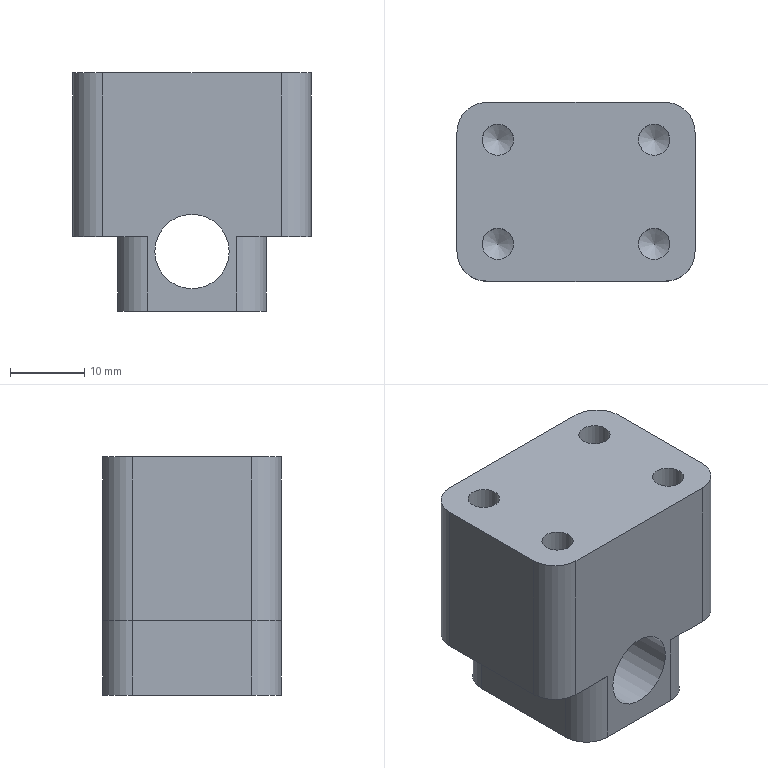Part | NX | features BREP 1, DATUM_CSYS 1 | 1 solid | 37 faces | box 32 x 24 x 32 mm | volume 18240 mm3 | cylinder 21 | plane 10 | cone 6 | commonest cylinder face diameters 4.2 x8 8 x8 2.5 x4 10 x1
STEP:
#1=CARTESIAN_POINT('',(12.,12.,5.));
#2=VERTEX_POINT('',#1);
#3=CARTESIAN_POINT('',(6.,12.,5.));
#4=VERTEX_POINT('',#3);
#5=CARTESIAN_POINT('',(12.,12.,5.));
#6=DIRECTION('',(-1.,0.,0.));
#7=VECTOR('',#6,1000.);
#8=LINE('',#5,#7);
#9=EDGE_CURVE('',#2,#4,#8,.T.);
#10=ORIENTED_EDGE('',*,*,#9,.T.);
#11=CARTESIAN_POINT('',(6.,12.,-5.));
#12=VERTEX_POINT('',#11);
#13=CARTESIAN_POINT('',(6.,12.,-5.));
#14=DIRECTION('',(0.,0.,1.));
#15=VECTOR('',#14,1000.);
#16=LINE('',#13,#15);
#17=EDGE_CURVE('',#12,#4,#16,.T.);
#18=ORIENTED_EDGE('',*,*,#17,.F.);
#19=CARTESIAN_POINT('',(-6.,12.,-5.));
#20=VERTEX_POINT('',#19);
#21=CARTESIAN_POINT('',(-6.,12.,-5.));
#22=DIRECTION('',(1.,0.,0.));
#23=VECTOR('',#22,1000.);
#24=LINE('',#21,#23);
#25=EDGE_CURVE('',#20,#12,#24,.T.);
#26=ORIENTED_EDGE('',*,*,#25,.F.);
#27=CARTESIAN_POINT('',(-6.,12.,5.));
#28=VERTEX_POINT('',#27);
#29=CARTESIAN_POINT('',(-6.,12.,5.));
#30=DIRECTION('',(0.,0.,-1.));
#31=VECTOR('',#30,1000.);
#32=LINE('',#29,#31);
#33=EDGE_CURVE('',#28,#20,#32,.T.);
#34=ORIENTED_EDGE('',*,*,#33,.F.);
#35=CARTESIAN_POINT('',(-12.,12.,5.));
#36=VERTEX_POINT('',#35);
#37=CARTESIAN_POINT('',(-12.,12.,5.));
#38=DIRECTION('',(1.,0.,0.));
#39=VECTOR('',#38,1000.);
#40=LINE('',#37,#39);
#41=EDGE_CURVE('',#36,#28,#40,.T.);
#42=ORIENTED_EDGE('',*,*,#41,.F.);
#43=CARTESIAN_POINT('',(-12.,12.,27.));
#44=VERTEX_POINT('',#43);
#45=CARTESIAN_POINT('',(-12.,12.,27.));
#46=DIRECTION('',(0.,0.,-1.));
#47=VECTOR('',#46,1000.);
#48=LINE('',#45,#47);
#49=EDGE_CURVE('',#44,#36,#48,.T.);
#50=ORIENTED_EDGE('',*,*,#49,.F.);
#51=CARTESIAN_POINT('',(12.,12.,27.));
#52=VERTEX_POINT('',#51);
#53=CARTESIAN_POINT('',(12.,12.,27.));
#54=DIRECTION('',(-1.,0.,0.));
#55=VECTOR('',#54,1000.);
#56=LINE('',#53,#55);
#57=EDGE_CURVE('',#52,#44,#56,.T.);
#58=ORIENTED_EDGE('',*,*,#57,.F.);
#59=CARTESIAN_POINT('',(12.,12.,5.));
#60=DIRECTION('',(0.,0.,1.));
#61=VECTOR('',#60,1000.);
#62=LINE('',#59,#61);
#63=EDGE_CURVE('',#2,#52,#62,.T.);
#64=ORIENTED_EDGE('',*,*,#63,.F.);
#65=EDGE_LOOP('',(#10,#18,#26,#34,#42,#50,#58,#64));
#66=FACE_BOUND('',#65,.T.);
#67=CARTESIAN_POINT('',(5.,12.,3.));
#68=VERTEX_POINT('',#67);
#69=CARTESIAN_POINT('',(0.,12.,3.));
#70=DIRECTION('',(0.,1.,0.));
#71=DIRECTION('',(1.,0.,0.));
#72=AXIS2_PLACEMENT_3D('',#69,#70,#71);
#73=CIRCLE('',#72,5.);
#74=EDGE_CURVE('',#68,#68,#73,.T.);
#75=ORIENTED_EDGE('',*,*,#74,.F.);
#76=EDGE_LOOP('',(#75));
#77=FACE_BOUND('',#76,.T.);
#78=CARTESIAN_POINT('',(0.,12.,11.));
#79=DIRECTION('',(0.,-1.,0.));
#80=DIRECTION('',(-1.,0.,0.));
#81=AXIS2_PLACEMENT_3D('',#78,#79,#80);
#82=PLANE('',#81);
#83=ADVANCED_FACE('',(#66,#77),#82,.F.);
#84=CARTESIAN_POINT('',(12.,-12.,5.));
#85=VERTEX_POINT('',#84);
#86=CARTESIAN_POINT('',(12.,-12.,27.));
#87=VERTEX_POINT('',#86);
#88=CARTESIAN_POINT('',(12.,-12.,5.));
#89=DIRECTION('',(0.,0.,1.));
#90=VECTOR('',#89,1000.);
#91=LINE('',#88,#90);
#92=EDGE_CURVE('',#85,#87,#91,.T.);
#93=ORIENTED_EDGE('',*,*,#92,.T.);
#94=CARTESIAN_POINT('',(-12.,-12.,27.));
#95=VERTEX_POINT('',#94);
#96=CARTESIAN_POINT('',(12.,-12.,27.));
#97=DIRECTION('',(-1.,0.,0.));
#98=VECTOR('',#97,1000.);
#99=LINE('',#96,#98);
#100=EDGE_CURVE('',#87,#95,#99,.T.);
#101=ORIENTED_EDGE('',*,*,#100,.T.);
#102=CARTESIAN_POINT('',(-12.,-12.,5.));
#103=VERTEX_POINT('',#102);
#104=CARTESIAN_POINT('',(-12.,-12.,27.));
#105=DIRECTION('',(0.,0.,-1.));
#106=VECTOR('',#105,1000.);
#107=LINE('',#104,#106);
#108=EDGE_CURVE('',#95,#103,#107,.T.);
#109=ORIENTED_EDGE('',*,*,#108,.T.);
#110=CARTESIAN_POINT('',(-6.,-12.,5.));
#111=VERTEX_POINT('',#110);
#112=CARTESIAN_POINT('',(-12.,-12.,5.));
#113=DIRECTION('',(1.,0.,0.));
#114=VECTOR('',#113,1000.);
#115=LINE('',#112,#114);
#116=EDGE_CURVE('',#103,#111,#115,.T.);
#117=ORIENTED_EDGE('',*,*,#116,.T.);
#118=CARTESIAN_POINT('',(-6.,-12.,-5.));
#119=VERTEX_POINT('',#118);
#120=CARTESIAN_POINT('',(-6.,-12.,5.));
#121=DIRECTION('',(0.,0.,-1.));
#122=VECTOR('',#121,1000.);
#123=LINE('',#120,#122);
#124=EDGE_CURVE('',#111,#119,#123,.T.);
#125=ORIENTED_EDGE('',*,*,#124,.T.);
#126=CARTESIAN_POINT('',(6.,-12.,-5.));
#127=VERTEX_POINT('',#126);
#128=CARTESIAN_POINT('',(-6.,-12.,-5.));
#129=DIRECTION('',(1.,0.,0.));
#130=VECTOR('',#129,1000.);
#131=LINE('',#128,#130);
#132=EDGE_CURVE('',#119,#127,#131,.T.);
#133=ORIENTED_EDGE('',*,*,#132,.T.);
#134=CARTESIAN_POINT('',(6.,-12.,5.));
#135=VERTEX_POINT('',#134);
#136=CARTESIAN_POINT('',(6.,-12.,-5.));
#137=DIRECTION('',(0.,0.,1.));
#138=VECTOR('',#137,1000.);
#139=LINE('',#136,#138);
#140=EDGE_CURVE('',#127,#135,#139,.T.);
#141=ORIENTED_EDGE('',*,*,#140,.T.);
#142=CARTESIAN_POINT('',(12.,-12.,5.));
#143=DIRECTION('',(-1.,0.,0.));
#144=VECTOR('',#143,1000.);
#145=LINE('',#142,#144);
#146=EDGE_CURVE('',#85,#135,#145,.T.);
#147=ORIENTED_EDGE('',*,*,#146,.F.);
#148=EDGE_LOOP('',(#93,#101,#109,#117,#125,#133,#141,#147));
#149=FACE_BOUND('',#148,.T.);
#150=CARTESIAN_POINT('',(5.,-12.,3.));
#151=VERTEX_POINT('',#150);
#152=CARTESIAN_POINT('',(0.,-12.,3.));
#153=DIRECTION('',(0.,1.,0.));
#154=DIRECTION('',(1.,0.,0.));
#155=AXIS2_PLACEMENT_3D('',#152,#153,#154);
#156=CIRCLE('',#155,5.);
#157=EDGE_CURVE('',#151,#151,#156,.T.);
#158=ORIENTED_EDGE('',*,*,#157,.T.);
#159=EDGE_LOOP('',(#158));
#160=FACE_BOUND('',#159,.T.);
#161=CARTESIAN_POINT('',(0.,-12.,11.));
#162=DIRECTION('',(0.,-1.,0.));
#163=DIRECTION('',(-1.,0.,0.));
#164=AXIS2_PLACEMENT_3D('',#161,#162,#163);
#165=PLANE('',#164);
#166=ADVANCED_FACE('',(#149,#160),#165,.T.);
#167=ORIENTED_EDGE('',*,*,#25,.T.);
#168=CARTESIAN_POINT('',(10.,8.,-5.));
#169=VERTEX_POINT('',#168);
#170=CARTESIAN_POINT('',(6.,8.,-5.));
#171=DIRECTION('',(0.,0.,-1.));
#172=DIRECTION('',(0.,1.,0.));
#173=AXIS2_PLACEMENT_3D('',#170,#171,#172);
#174=CIRCLE('',#173,4.);
#175=EDGE_CURVE('',#12,#169,#174,.T.);
#176=ORIENTED_EDGE('',*,*,#175,.T.);
#177=CARTESIAN_POINT('',(10.,-8.,-5.));
#178=VERTEX_POINT('',#177);
#179=CARTESIAN_POINT('',(10.,8.,-5.));
#180=DIRECTION('',(0.,-1.,0.));
#181=VECTOR('',#180,1000.);
#182=LINE('',#179,#181);
#183=EDGE_CURVE('',#169,#178,#182,.T.);
#184=ORIENTED_EDGE('',*,*,#183,.T.);
#185=CARTESIAN_POINT('',(6.,-8.,-5.));
#186=DIRECTION('',(0.,0.,1.));
#187=DIRECTION('',(0.,-1.,0.));
#188=AXIS2_PLACEMENT_3D('',#185,#186,#187);
#189=CIRCLE('',#188,4.);
#190=EDGE_CURVE('',#127,#178,#189,.T.);
#191=ORIENTED_EDGE('',*,*,#190,.F.);
#192=ORIENTED_EDGE('',*,*,#132,.F.);
#193=CARTESIAN_POINT('',(-10.,-8.,-5.));
#194=VERTEX_POINT('',#193);
#195=CARTESIAN_POINT('',(-6.,-8.,-5.));
#196=DIRECTION('',(0.,0.,-1.));
#197=DIRECTION('',(0.,-1.,0.));
#198=AXIS2_PLACEMENT_3D('',#195,#196,#197);
#199=CIRCLE('',#198,4.);
#200=EDGE_CURVE('',#119,#194,#199,.T.);
#201=ORIENTED_EDGE('',*,*,#200,.T.);
#202=CARTESIAN_POINT('',(-10.,8.,-5.));
#203=VERTEX_POINT('',#202);
#204=CARTESIAN_POINT('',(-10.,8.,-5.));
#205=DIRECTION('',(0.,-1.,0.));
#206=VECTOR('',#205,1000.);
#207=LINE('',#204,#206);
#208=EDGE_CURVE('',#203,#194,#207,.T.);
#209=ORIENTED_EDGE('',*,*,#208,.F.);
#210=CARTESIAN_POINT('',(-6.,8.,-5.));
#211=DIRECTION('',(0.,0.,1.));
#212=DIRECTION('',(0.,1.,0.));
#213=AXIS2_PLACEMENT_3D('',#210,#211,#212);
#214=CIRCLE('',#213,4.);
#215=EDGE_CURVE('',#20,#203,#214,.T.);
#216=ORIENTED_EDGE('',*,*,#215,.F.);
#217=EDGE_LOOP('',(#167,#176,#184,#191,#192,#201,#209,#216));
#218=FACE_BOUND('',#217,.T.);
#219=CARTESIAN_POINT('',(8.75,0.,-5.));
#220=VERTEX_POINT('',#219);
#221=CARTESIAN_POINT('',(7.5,0.,-5.));
#222=DIRECTION('',(0.,0.,1.));
#223=DIRECTION('',(1.,0.,0.));
#224=AXIS2_PLACEMENT_3D('',#221,#222,#223);
#225=CIRCLE('',#224,1.25);
#226=EDGE_CURVE('',#220,#220,#225,.T.);
#227=ORIENTED_EDGE('',*,*,#226,.T.);
#228=EDGE_LOOP('',(#227));
#229=FACE_BOUND('',#228,.T.);
#230=CARTESIAN_POINT('',(-6.25,0.,-5.));
#231=VERTEX_POINT('',#230);
#232=CARTESIAN_POINT('',(-7.5,0.,-5.));
#233=DIRECTION('',(0.,0.,1.));
#234=DIRECTION('',(1.,0.,0.));
#235=AXIS2_PLACEMENT_3D('',#232,#233,#234);
#236=CIRCLE('',#235,1.25);
#237=EDGE_CURVE('',#231,#231,#236,.T.);
#238=ORIENTED_EDGE('',*,*,#237,.T.);
#239=EDGE_LOOP('',(#238));
#240=FACE_BOUND('',#239,.T.);
#241=CARTESIAN_POINT('',(0.,0.,-5.));
#242=DIRECTION('',(0.,0.,-1.));
#243=DIRECTION('',(-1.,0.,0.));
#244=AXIS2_PLACEMENT_3D('',#241,#242,#243);
#245=PLANE('',#244);
#246=ADVANCED_FACE('',(#218,#229,#240),#245,.T.);
#247=ORIENTED_EDGE('',*,*,#183,.F.);
#248=CARTESIAN_POINT('',(10.,8.,5.));
#249=VERTEX_POINT('',#248);
#250=CARTESIAN_POINT('',(10.,8.,-5.));
#251=DIRECTION('',(0.,0.,1.));
#252=VECTOR('',#251,1000.);
#253=LINE('',#250,#252);
#254=EDGE_CURVE('',#169,#249,#253,.T.);
#255=ORIENTED_EDGE('',*,*,#254,.T.);
#256=CARTESIAN_POINT('',(10.,-8.,5.));
#257=VERTEX_POINT('',#256);
#258=CARTESIAN_POINT('',(10.,8.,5.));
#259=DIRECTION('',(0.,-1.,0.));
#260=VECTOR('',#259,1000.);
#261=LINE('',#258,#260);
#262=EDGE_CURVE('',#249,#257,#261,.T.);
#263=ORIENTED_EDGE('',*,*,#262,.T.);
#264=CARTESIAN_POINT('',(10.,-8.,-5.));
#265=DIRECTION('',(0.,0.,1.));
#266=VECTOR('',#265,1000.);
#267=LINE('',#264,#266);
#268=EDGE_CURVE('',#178,#257,#267,.T.);
#269=ORIENTED_EDGE('',*,*,#268,.F.);
#270=EDGE_LOOP('',(#247,#255,#263,#269));
#271=FACE_BOUND('',#270,.T.);
#272=CARTESIAN_POINT('',(10.,0.,0.));
#273=DIRECTION('',(1.,0.,0.));
#274=DIRECTION('',(0.,0.,-1.));
#275=AXIS2_PLACEMENT_3D('',#272,#273,#274);
#276=PLANE('',#275);
#277=ADVANCED_FACE('',(#271),#276,.T.);
#278=CARTESIAN_POINT('',(16.,8.,5.));
#279=VERTEX_POINT('',#278);
#280=CARTESIAN_POINT('',(12.,8.,5.));
#281=DIRECTION('',(0.,0.,-1.));
#282=DIRECTION('',(0.,1.,0.));
#283=AXIS2_PLACEMENT_3D('',#280,#281,#282);
#284=CIRCLE('',#283,4.);
#285=EDGE_CURVE('',#2,#279,#284,.T.);
#286=ORIENTED_EDGE('',*,*,#285,.T.);
#287=CARTESIAN_POINT('',(16.,-8.,5.));
#288=VERTEX_POINT('',#287);
#289=CARTESIAN_POINT('',(16.,8.,5.));
#290=DIRECTION('',(0.,-1.,0.));
#291=VECTOR('',#290,1000.);
#292=LINE('',#289,#291);
#293=EDGE_CURVE('',#279,#288,#292,.T.);
#294=ORIENTED_EDGE('',*,*,#293,.T.);
#295=CARTESIAN_POINT('',(12.,-8.,5.));
#296=DIRECTION('',(0.,0.,1.));
#297=DIRECTION('',(0.,-1.,0.));
#298=AXIS2_PLACEMENT_3D('',#295,#296,#297);
#299=CIRCLE('',#298,4.);
#300=EDGE_CURVE('',#85,#288,#299,.T.);
#301=ORIENTED_EDGE('',*,*,#300,.F.);
#302=ORIENTED_EDGE('',*,*,#146,.T.);
#303=CARTESIAN_POINT('',(6.,-8.,5.));
#304=DIRECTION('',(0.,0.,-1.));
#305=DIRECTION('',(1.,0.,0.));
#306=AXIS2_PLACEMENT_3D('',#303,#304,#305);
#307=CIRCLE('',#306,4.);
#308=EDGE_CURVE('',#257,#135,#307,.T.);
#309=ORIENTED_EDGE('',*,*,#308,.F.);
#310=ORIENTED_EDGE('',*,*,#262,.F.);
#311=CARTESIAN_POINT('',(6.,8.,5.));
#312=DIRECTION('',(0.,0.,1.));
#313=DIRECTION('',(1.,0.,0.));
#314=AXIS2_PLACEMENT_3D('',#311,#312,#313);
#315=CIRCLE('',#314,4.);
#316=EDGE_CURVE('',#249,#4,#315,.T.);
#317=ORIENTED_EDGE('',*,*,#316,.T.);
#318=ORIENTED_EDGE('',*,*,#9,.F.);
#319=EDGE_LOOP('',(#286,#294,#301,#302,#309,#310,#317,#318));
#320=FACE_BOUND('',#319,.T.);
#321=CARTESIAN_POINT('',(11.,0.,5.));
#322=DIRECTION('',(0.,0.,-1.));
#323=DIRECTION('',(-1.,0.,0.));
#324=AXIS2_PLACEMENT_3D('',#321,#322,#323);
#325=PLANE('',#324);
#326=ADVANCED_FACE('',(#320),#325,.T.);
#327=ORIENTED_EDGE('',*,*,#293,.F.);
#328=CARTESIAN_POINT('',(16.,8.,27.));
#329=VERTEX_POINT('',#328);
#330=CARTESIAN_POINT('',(16.,8.,5.));
#331=DIRECTION('',(0.,0.,1.));
#332=VECTOR('',#331,1000.);
#333=LINE('',#330,#332);
#334=EDGE_CURVE('',#279,#329,#333,.T.);
#335=ORIENTED_EDGE('',*,*,#334,.T.);
#336=CARTESIAN_POINT('',(16.,-8.,27.));
#337=VERTEX_POINT('',#336);
#338=CARTESIAN_POINT('',(16.,8.,27.));
#339=DIRECTION('',(0.,-1.,0.));
#340=VECTOR('',#339,1000.);
#341=LINE('',#338,#340);
#342=EDGE_CURVE('',#329,#337,#341,.T.);
#343=ORIENTED_EDGE('',*,*,#342,.T.);
#344=CARTESIAN_POINT('',(16.,-8.,5.));
#345=DIRECTION('',(0.,0.,1.));
#346=VECTOR('',#345,1000.);
#347=LINE('',#344,#346);
#348=EDGE_CURVE('',#288,#337,#347,.T.);
#349=ORIENTED_EDGE('',*,*,#348,.F.);
#350=EDGE_LOOP('',(#327,#335,#343,#349));
#351=FACE_BOUND('',#350,.T.);
#352=CARTESIAN_POINT('',(16.,0.,16.));
#353=DIRECTION('',(1.,0.,0.));
#354=DIRECTION('',(0.,0.,-1.));
#355=AXIS2_PLACEMENT_3D('',#352,#353,#354);
#356=PLANE('',#355);
#357=ADVANCED_FACE('',(#351),#356,.T.);
#358=CARTESIAN_POINT('',(-16.,8.,27.));
#359=VERTEX_POINT('',#358);
#360=CARTESIAN_POINT('',(-16.,-8.,27.));
#361=VERTEX_POINT('',#360);
#362=CARTESIAN_POINT('',(-16.,8.,27.));
#363=DIRECTION('',(0.,-1.,0.));
#364=VECTOR('',#363,1000.);
#365=LINE('',#362,#364);
#366=EDGE_CURVE('',#359,#361,#365,.T.);
#367=ORIENTED_EDGE('',*,*,#366,.F.);
#368=CARTESIAN_POINT('',(-16.,8.,5.));
#369=VERTEX_POINT('',#368);
#370=CARTESIAN_POINT('',(-16.,8.,27.));
#371=DIRECTION('',(0.,0.,-1.));
#372=VECTOR('',#371,1000.);
#373=LINE('',#370,#372);
#374=EDGE_CURVE('',#359,#369,#373,.T.);
#375=ORIENTED_EDGE('',*,*,#374,.T.);
#376=CARTESIAN_POINT('',(-16.,-8.,5.));
#377=VERTEX_POINT('',#376);
#378=CARTESIAN_POINT('',(-16.,8.,5.));
#379=DIRECTION('',(0.,-1.,0.));
#380=VECTOR('',#379,1000.);
#381=LINE('',#378,#380);
#382=EDGE_CURVE('',#369,#377,#381,.T.);
#383=ORIENTED_EDGE('',*,*,#382,.T.);
#384=CARTESIAN_POINT('',(-16.,-8.,27.));
#385=DIRECTION('',(0.,0.,-1.));
#386=VECTOR('',#385,1000.);
#387=LINE('',#384,#386);
#388=EDGE_CURVE('',#361,#377,#387,.T.);
#389=ORIENTED_EDGE('',*,*,#388,.F.);
#390=EDGE_LOOP('',(#367,#375,#383,#389));
#391=FACE_BOUND('',#390,.T.);
#392=CARTESIAN_POINT('',(-16.,0.,16.));
#393=DIRECTION('',(-1.,0.,0.));
#394=DIRECTION('',(0.,0.,1.));
#395=AXIS2_PLACEMENT_3D('',#392,#393,#394);
#396=PLANE('',#395);
#397=ADVANCED_FACE('',(#391),#396,.T.);
#398=CARTESIAN_POINT('',(-12.,-8.,5.));
#399=DIRECTION('',(0.,0.,-1.));
#400=DIRECTION('',(0.,-1.,0.));
#401=AXIS2_PLACEMENT_3D('',#398,#399,#400);
#402=CIRCLE('',#401,4.);
#403=EDGE_CURVE('',#103,#377,#402,.T.);
#404=ORIENTED_EDGE('',*,*,#403,.T.);
#405=ORIENTED_EDGE('',*,*,#382,.F.);
#406=CARTESIAN_POINT('',(-12.,8.,5.));
#407=DIRECTION('',(0.,0.,1.));
#408=DIRECTION('',(0.,1.,0.));
#409=AXIS2_PLACEMENT_3D('',#406,#407,#408);
#410=CIRCLE('',#409,4.);
#411=EDGE_CURVE('',#36,#369,#410,.T.);
#412=ORIENTED_EDGE('',*,*,#411,.F.);
#413=ORIENTED_EDGE('',*,*,#41,.T.);
#414=CARTESIAN_POINT('',(-10.,8.,5.));
#415=VERTEX_POINT('',#414);
#416=CARTESIAN_POINT('',(-6.,8.,5.));
#417=DIRECTION('',(0.,0.,-1.));
#418=DIRECTION('',(-1.,0.,0.));
#419=AXIS2_PLACEMENT_3D('',#416,#417,#418);
#420=CIRCLE('',#419,4.);
#421=EDGE_CURVE('',#415,#28,#420,.T.);
#422=ORIENTED_EDGE('',*,*,#421,.F.);
#423=CARTESIAN_POINT('',(-10.,-8.,5.));
#424=VERTEX_POINT('',#423);
#425=CARTESIAN_POINT('',(-10.,8.,5.));
#426=DIRECTION('',(0.,-1.,0.));
#427=VECTOR('',#426,1000.);
#428=LINE('',#425,#427);
#429=EDGE_CURVE('',#415,#424,#428,.T.);
#430=ORIENTED_EDGE('',*,*,#429,.T.);
#431=CARTESIAN_POINT('',(-6.,-8.,5.));
#432=DIRECTION('',(0.,0.,1.));
#433=DIRECTION('',(-1.,0.,0.));
#434=AXIS2_PLACEMENT_3D('',#431,#432,#433);
#435=CIRCLE('',#434,4.);
#436=EDGE_CURVE('',#424,#111,#435,.T.);
#437=ORIENTED_EDGE('',*,*,#436,.T.);
#438=ORIENTED_EDGE('',*,*,#116,.F.);
#439=EDGE_LOOP('',(#404,#405,#412,#413,#422,#430,#437,#438));
#440=FACE_BOUND('',#439,.T.);
#441=CARTESIAN_POINT('',(-11.,0.,5.));
#442=DIRECTION('',(0.,0.,-1.));
#443=DIRECTION('',(-1.,0.,0.));
#444=AXIS2_PLACEMENT_3D('',#441,#442,#443);
#445=PLANE('',#444);
#446=ADVANCED_FACE('',(#440),#445,.T.);
#447=ORIENTED_EDGE('',*,*,#429,.F.);
#448=CARTESIAN_POINT('',(-10.,8.,5.));
#449=DIRECTION('',(0.,0.,-1.));
#450=VECTOR('',#449,1000.);
#451=LINE('',#448,#450);
#452=EDGE_CURVE('',#415,#203,#451,.T.);
#453=ORIENTED_EDGE('',*,*,#452,.T.);
#454=ORIENTED_EDGE('',*,*,#208,.T.);
#455=CARTESIAN_POINT('',(-10.,-8.,5.));
#456=DIRECTION('',(0.,0.,-1.));
#457=VECTOR('',#456,1000.);
#458=LINE('',#455,#457);
#459=EDGE_CURVE('',#424,#194,#458,.T.);
#460=ORIENTED_EDGE('',*,*,#459,.F.);
#461=EDGE_LOOP('',(#447,#453,#454,#460));
#462=FACE_BOUND('',#461,.T.);
#463=CARTESIAN_POINT('',(-10.,0.,0.));
#464=DIRECTION('',(-1.,0.,0.));
#465=DIRECTION('',(0.,0.,1.));
#466=AXIS2_PLACEMENT_3D('',#463,#464,#465);
#467=PLANE('',#466);
#468=ADVANCED_FACE('',(#462),#467,.T.);
#469=CARTESIAN_POINT('',(12.,-8.,27.));
#470=DIRECTION('',(0.,0.,1.));
#471=DIRECTION('',(0.,-1.,0.));
#472=AXIS2_PLACEMENT_3D('',#469,#470,#471);
#473=CIRCLE('',#472,4.);
#474=EDGE_CURVE('',#87,#337,#473,.T.);
#475=ORIENTED_EDGE('',*,*,#474,.F.);
#476=ORIENTED_EDGE('',*,*,#92,.F.);
#477=ORIENTED_EDGE('',*,*,#300,.T.);
#478=ORIENTED_EDGE('',*,*,#348,.T.);
#479=EDGE_LOOP('',(#475,#476,#477,#478));
#480=FACE_BOUND('',#479,.T.);
#481=CARTESIAN_POINT('',(12.,-8.,-6.117));
#482=DIRECTION('',(0.,0.,1.));
#483=DIRECTION('',(0.,1.,0.));
#484=AXIS2_PLACEMENT_3D('',#481,#482,#483);
#485=CYLINDRICAL_SURFACE('',#484,4.);
#486=ADVANCED_FACE('',(#480),#485,.T.);
#487=CARTESIAN_POINT('',(-12.,-8.,27.));
#488=DIRECTION('',(0.,0.,-1.));
#489=DIRECTION('',(0.,-1.,0.));
#490=AXIS2_PLACEMENT_3D('',#487,#488,#489);
#491=CIRCLE('',#490,4.);
#492=EDGE_CURVE('',#95,#361,#491,.T.);
#493=ORIENTED_EDGE('',*,*,#492,.T.);
#494=ORIENTED_EDGE('',*,*,#388,.T.);
#495=ORIENTED_EDGE('',*,*,#403,.F.);
#496=ORIENTED_EDGE('',*,*,#108,.F.);
#497=EDGE_LOOP('',(#493,#494,#495,#496));
#498=FACE_BOUND('',#497,.T.);
#499=CARTESIAN_POINT('',(-12.,-8.,27.));
#500=DIRECTION('',(0.,0.,-1.));
#501=DIRECTION('',(0.,1.,0.));
#502=AXIS2_PLACEMENT_3D('',#499,#500,#501);
#503=CYLINDRICAL_SURFACE('',#502,4.);
#504=ADVANCED_FACE('',(#498),#503,.T.);
#505=ORIENTED_EDGE('',*,*,#334,.F.);
#506=ORIENTED_EDGE('',*,*,#285,.F.);
#507=ORIENTED_EDGE('',*,*,#63,.T.);
#508=CARTESIAN_POINT('',(12.,8.,27.));
#509=DIRECTION('',(0.,0.,-1.));
#510=DIRECTION('',(0.,1.,0.));
#511=AXIS2_PLACEMENT_3D('',#508,#509,#510);
#512=CIRCLE('',#511,4.);
#513=EDGE_CURVE('',#52,#329,#512,.T.);
#514=ORIENTED_EDGE('',*,*,#513,.T.);
#515=EDGE_LOOP('',(#505,#506,#507,#514));
#516=FACE_BOUND('',#515,.T.);
#517=CARTESIAN_POINT('',(12.,8.,-6.6));
#518=DIRECTION('',(0.,0.,1.));
#519=DIRECTION('',(0.,-1.,0.));
#520=AXIS2_PLACEMENT_3D('',#517,#518,#519);
#521=CYLINDRICAL_SURFACE('',#520,4.);
#522=ADVANCED_FACE('',(#516),#521,.T.);
#523=ORIENTED_EDGE('',*,*,#49,.T.);
#524=ORIENTED_EDGE('',*,*,#411,.T.);
#525=ORIENTED_EDGE('',*,*,#374,.F.);
#526=CARTESIAN_POINT('',(-12.,8.,27.));
#527=DIRECTION('',(0.,0.,1.));
#528=DIRECTION('',(0.,1.,0.));
#529=AXIS2_PLACEMENT_3D('',#526,#527,#528);
#530=CIRCLE('',#529,4.);
#531=EDGE_CURVE('',#44,#359,#530,.T.);
#532=ORIENTED_EDGE('',*,*,#531,.F.);
#533=EDGE_LOOP('',(#523,#524,#525,#532));
#534=FACE_BOUND('',#533,.T.);
#535=CARTESIAN_POINT('',(-12.,8.,27.));
#536=DIRECTION('',(0.,0.,-1.));
#537=DIRECTION('',(0.,-1.,0.));
#538=AXIS2_PLACEMENT_3D('',#535,#536,#537);
#539=CYLINDRICAL_SURFACE('',#538,4.);
#540=ADVANCED_FACE('',(#534),#539,.T.);
#541=ORIENTED_EDGE('',*,*,#452,.F.);
#542=ORIENTED_EDGE('',*,*,#421,.T.);
#543=ORIENTED_EDGE('',*,*,#33,.T.);
#544=ORIENTED_EDGE('',*,*,#215,.T.);
#545=EDGE_LOOP('',(#541,#542,#543,#544));
#546=FACE_BOUND('',#545,.T.);
#547=CARTESIAN_POINT('',(-6.,8.,28.175));
#548=DIRECTION('',(0.,0.,-1.));
#549=DIRECTION('',(0.,-1.,0.));
#550=AXIS2_PLACEMENT_3D('',#547,#548,#549);
#551=CYLINDRICAL_SURFACE('',#550,4.);
#552=ADVANCED_FACE('',(#546),#551,.T.);
#553=ORIENTED_EDGE('',*,*,#17,.T.);
#554=ORIENTED_EDGE('',*,*,#316,.F.);
#555=ORIENTED_EDGE('',*,*,#254,.F.);
#556=ORIENTED_EDGE('',*,*,#175,.F.);
#557=EDGE_LOOP('',(#553,#554,#555,#556));
#558=FACE_BOUND('',#557,.T.);
#559=CARTESIAN_POINT('',(6.,8.,-5.));
#560=DIRECTION('',(0.,0.,1.));
#561=DIRECTION('',(0.,-1.,0.));
#562=AXIS2_PLACEMENT_3D('',#559,#560,#561);
#563=CYLINDRICAL_SURFACE('',#562,4.);
#564=ADVANCED_FACE('',(#558),#563,.T.);
#565=ORIENTED_EDGE('',*,*,#190,.T.);
#566=ORIENTED_EDGE('',*,*,#268,.T.);
#567=ORIENTED_EDGE('',*,*,#308,.T.);
#568=ORIENTED_EDGE('',*,*,#140,.F.);
#569=EDGE_LOOP('',(#565,#566,#567,#568));
#570=FACE_BOUND('',#569,.T.);
#571=CARTESIAN_POINT('',(6.,-8.,-5.));
#572=DIRECTION('',(0.,0.,1.));
#573=DIRECTION('',(0.,1.,0.));
#574=AXIS2_PLACEMENT_3D('',#571,#572,#573);
#575=CYLINDRICAL_SURFACE('',#574,4.);
#576=ADVANCED_FACE('',(#570),#575,.T.);
#577=ORIENTED_EDGE('',*,*,#200,.F.);
#578=ORIENTED_EDGE('',*,*,#124,.F.);
#579=ORIENTED_EDGE('',*,*,#436,.F.);
#580=ORIENTED_EDGE('',*,*,#459,.T.);
#581=EDGE_LOOP('',(#577,#578,#579,#580));
#582=FACE_BOUND('',#581,.T.);
#583=CARTESIAN_POINT('',(-6.,-8.,28.6));
#584=DIRECTION('',(0.,0.,-1.));
#585=DIRECTION('',(0.,1.,0.));
#586=AXIS2_PLACEMENT_3D('',#583,#584,#585);
#587=CYLINDRICAL_SURFACE('',#586,4.);
#588=ADVANCED_FACE('',(#582),#587,.T.);
#589=ORIENTED_EDGE('',*,*,#100,.F.);
#590=ORIENTED_EDGE('',*,*,#474,.T.);
#591=ORIENTED_EDGE('',*,*,#342,.F.);
#592=ORIENTED_EDGE('',*,*,#513,.F.);
#593=ORIENTED_EDGE('',*,*,#57,.T.);
#594=ORIENTED_EDGE('',*,*,#531,.T.);
#595=ORIENTED_EDGE('',*,*,#366,.T.);
#596=ORIENTED_EDGE('',*,*,#492,.F.);
#597=EDGE_LOOP('',(#589,#590,#591,#592,#593,#594,#595,#596));
#598=FACE_BOUND('',#597,.T.);
#599=CARTESIAN_POINT('',(-8.4,7.,27.));
#600=VERTEX_POINT('',#599);
#601=CARTESIAN_POINT('',(-10.5,7.,27.));
#602=DIRECTION('',(0.,0.,-1.));
#603=DIRECTION('',(1.,0.,0.));
#604=AXIS2_PLACEMENT_3D('',#601,#602,#603);
#605=CIRCLE('',#604,2.1);
#606=EDGE_CURVE('',#600,#600,#605,.T.);
#607=ORIENTED_EDGE('',*,*,#606,.T.);
#608=EDGE_LOOP('',(#607));
#609=FACE_BOUND('',#608,.T.);
#610=CARTESIAN_POINT('',(12.6,7.,27.));
#611=VERTEX_POINT('',#610);
#612=CARTESIAN_POINT('',(10.5,7.,27.));
#613=DIRECTION('',(0.,0.,-1.));
#614=DIRECTION('',(1.,0.,0.));
#615=AXIS2_PLACEMENT_3D('',#612,#613,#614);
#616=CIRCLE('',#615,2.1);
#617=EDGE_CURVE('',#611,#611,#616,.T.);
#618=ORIENTED_EDGE('',*,*,#617,.T.);
#619=EDGE_LOOP('',(#618));
#620=FACE_BOUND('',#619,.T.);
#621=CARTESIAN_POINT('',(12.6,-7.,27.));
#622=VERTEX_POINT('',#621);
#623=CARTESIAN_POINT('',(10.5,-7.,27.));
#624=DIRECTION('',(0.,0.,-1.));
#625=DIRECTION('',(1.,0.,0.));
#626=AXIS2_PLACEMENT_3D('',#623,#624,#625);
#627=CIRCLE('',#626,2.1);
#628=EDGE_CURVE('',#622,#622,#627,.T.);
#629=ORIENTED_EDGE('',*,*,#628,.T.);
#630=EDGE_LOOP('',(#629));
#631=FACE_BOUND('',#630,.T.);
#632=CARTESIAN_POINT('',(-8.4,-7.,27.));
#633=VERTEX_POINT('',#632);
#634=CARTESIAN_POINT('',(-10.5,-7.,27.));
#635=DIRECTION('',(0.,0.,-1.));
#636=DIRECTION('',(1.,0.,0.));
#637=AXIS2_PLACEMENT_3D('',#634,#635,#636);
#638=CIRCLE('',#637,2.1);
#639=EDGE_CURVE('',#633,#633,#638,.T.);
#640=ORIENTED_EDGE('',*,*,#639,.T.);
#641=EDGE_LOOP('',(#640));
#642=FACE_BOUND('',#641,.T.);
#643=CARTESIAN_POINT('',(0.,0.,27.));
#644=DIRECTION('',(0.,0.,1.));
#645=DIRECTION('',(1.,0.,0.));
#646=AXIS2_PLACEMENT_3D('',#643,#644,#645);
#647=PLANE('',#646);
#648=ADVANCED_FACE('',(#598,#609,#620,#631,#642),#647,.T.);
#649=CARTESIAN_POINT('',(-8.4,7.,11.));
#650=VERTEX_POINT('',#649);
#651=CARTESIAN_POINT('',(-8.4,7.,27.));
#652=DIRECTION('',(0.,0.,-1.));
#653=VECTOR('',#652,1000.);
#654=LINE('',#651,#653);
#655=EDGE_CURVE('',#600,#650,#654,.T.);
#656=ORIENTED_EDGE('',*,*,#655,.T.);
#657=CARTESIAN_POINT('',(-10.5,7.,11.));
#658=DIRECTION('',(0.,0.,-1.));
#659=DIRECTION('',(1.,0.,0.));
#660=AXIS2_PLACEMENT_3D('',#657,#658,#659);
#661=CIRCLE('',#660,2.1);
#662=EDGE_CURVE('',#650,#650,#661,.T.);
#663=ORIENTED_EDGE('',*,*,#662,.T.);
#664=ORIENTED_EDGE('',*,*,#655,.F.);
#665=ORIENTED_EDGE('',*,*,#606,.F.);
#666=EDGE_LOOP('',(#656,#663,#664,#665));
#667=FACE_BOUND('',#666,.T.);
#668=CARTESIAN_POINT('',(-10.5,7.,27.));
#669=DIRECTION('',(0.,0.,-1.));
#670=DIRECTION('',(-1.,0.,0.));
#671=AXIS2_PLACEMENT_3D('',#668,#669,#670);
#672=CYLINDRICAL_SURFACE('',#671,2.1);
#673=ADVANCED_FACE('',(#667),#672,.F.);
#674=CARTESIAN_POINT('',(12.6,7.,11.));
#675=VERTEX_POINT('',#674);
#676=CARTESIAN_POINT('',(12.6,7.,27.));
#677=DIRECTION('',(0.,0.,-1.));
#678=VECTOR('',#677,1000.);
#679=LINE('',#676,#678);
#680=EDGE_CURVE('',#611,#675,#679,.T.);
#681=ORIENTED_EDGE('',*,*,#680,.T.);
#682=CARTESIAN_POINT('',(10.5,7.,11.));
#683=DIRECTION('',(0.,0.,-1.));
#684=DIRECTION('',(1.,0.,0.));
#685=AXIS2_PLACEMENT_3D('',#682,#683,#684);
#686=CIRCLE('',#685,2.1);
#687=EDGE_CURVE('',#675,#675,#686,.T.);
#688=ORIENTED_EDGE('',*,*,#687,.T.);
#689=ORIENTED_EDGE('',*,*,#680,.F.);
#690=ORIENTED_EDGE('',*,*,#617,.F.);
#691=EDGE_LOOP('',(#681,#688,#689,#690));
#692=FACE_BOUND('',#691,.T.);
#693=CARTESIAN_POINT('',(10.5,7.,27.));
#694=DIRECTION('',(0.,0.,-1.));
#695=DIRECTION('',(-1.,0.,0.));
#696=AXIS2_PLACEMENT_3D('',#693,#694,#695);
#697=CYLINDRICAL_SURFACE('',#696,2.1);
#698=ADVANCED_FACE('',(#692),#697,.F.);
#699=CARTESIAN_POINT('',(12.6,-7.,11.));
#700=VERTEX_POINT('',#699);
#701=CARTESIAN_POINT('',(12.6,-7.,27.));
#702=DIRECTION('',(0.,0.,-1.));
#703=VECTOR('',#702,1000.);
#704=LINE('',#701,#703);
#705=EDGE_CURVE('',#622,#700,#704,.T.);
#706=ORIENTED_EDGE('',*,*,#705,.T.);
#707=CARTESIAN_POINT('',(10.5,-7.,11.));
#708=DIRECTION('',(0.,0.,-1.));
#709=DIRECTION('',(1.,0.,0.));
#710=AXIS2_PLACEMENT_3D('',#707,#708,#709);
#711=CIRCLE('',#710,2.1);
#712=EDGE_CURVE('',#700,#700,#711,.T.);
#713=ORIENTED_EDGE('',*,*,#712,.T.);
#714=ORIENTED_EDGE('',*,*,#705,.F.);
#715=ORIENTED_EDGE('',*,*,#628,.F.);
#716=EDGE_LOOP('',(#706,#713,#714,#715));
#717=FACE_BOUND('',#716,.T.);
#718=CARTESIAN_POINT('',(10.5,-7.,27.));
#719=DIRECTION('',(0.,0.,-1.));
#720=DIRECTION('',(-1.,0.,0.));
#721=AXIS2_PLACEMENT_3D('',#718,#719,#720);
#722=CYLINDRICAL_SURFACE('',#721,2.1);
#723=ADVANCED_FACE('',(#717),#722,.F.);
#724=CARTESIAN_POINT('',(-8.4,-7.,11.));
#725=VERTEX_POINT('',#724);
#726=CARTESIAN_POINT('',(-8.4,-7.,27.));
#727=DIRECTION('',(0.,0.,-1.));
#728=VECTOR('',#727,1000.);
#729=LINE('',#726,#728);
#730=EDGE_CURVE('',#633,#725,#729,.T.);
#731=ORIENTED_EDGE('',*,*,#730,.T.);
#732=CARTESIAN_POINT('',(-10.5,-7.,11.));
#733=DIRECTION('',(0.,0.,-1.));
#734=DIRECTION('',(1.,0.,0.));
#735=AXIS2_PLACEMENT_3D('',#732,#733,#734);
#736=CIRCLE('',#735,2.1);
#737=EDGE_CURVE('',#725,#725,#736,.T.);
#738=ORIENTED_EDGE('',*,*,#737,.T.);
#739=ORIENTED_EDGE('',*,*,#730,.F.);
#740=ORIENTED_EDGE('',*,*,#639,.F.);
#741=EDGE_LOOP('',(#731,#738,#739,#740));
#742=FACE_BOUND('',#741,.T.);
#743=CARTESIAN_POINT('',(-10.5,-7.,27.));
#744=DIRECTION('',(0.,0.,-1.));
#745=DIRECTION('',(-1.,0.,0.));
#746=AXIS2_PLACEMENT_3D('',#743,#744,#745);
#747=CYLINDRICAL_SURFACE('',#746,2.1);
#748=ADVANCED_FACE('',(#742),#747,.F.);
#749=CARTESIAN_POINT('',(-8.4,7.,9.));
#750=VERTEX_POINT('',#749);
#751=CARTESIAN_POINT('',(-8.4,7.,11.));
#752=DIRECTION('',(0.,0.,-1.));
#753=VECTOR('',#752,1000.);
#754=LINE('',#751,#753);
#755=EDGE_CURVE('',#650,#750,#754,.T.);
#756=ORIENTED_EDGE('',*,*,#755,.T.);
#757=CARTESIAN_POINT('',(-10.5,7.,9.));
#758=DIRECTION('',(0.,0.,-1.));
#759=DIRECTION('',(1.,0.,0.));
#760=AXIS2_PLACEMENT_3D('',#757,#758,#759);
#761=CIRCLE('',#760,2.1);
#762=EDGE_CURVE('',#750,#750,#761,.T.);
#763=ORIENTED_EDGE('',*,*,#762,.T.);
#764=ORIENTED_EDGE('',*,*,#755,.F.);
#765=ORIENTED_EDGE('',*,*,#662,.F.);
#766=EDGE_LOOP('',(#756,#763,#764,#765));
#767=FACE_BOUND('',#766,.T.);
#768=CARTESIAN_POINT('',(-10.5,7.,11.));
#769=DIRECTION('',(0.,0.,-1.));
#770=DIRECTION('',(-1.,0.,0.));
#771=AXIS2_PLACEMENT_3D('',#768,#769,#770);
#772=CYLINDRICAL_SURFACE('',#771,2.1);
#773=ADVANCED_FACE('',(#767),#772,.F.);
#774=CARTESIAN_POINT('',(12.6,7.,9.));
#775=VERTEX_POINT('',#774);
#776=CARTESIAN_POINT('',(12.6,7.,11.));
#777=DIRECTION('',(0.,0.,-1.));
#778=VECTOR('',#777,1000.);
#779=LINE('',#776,#778);
#780=EDGE_CURVE('',#675,#775,#779,.T.);
#781=ORIENTED_EDGE('',*,*,#780,.T.);
#782=CARTESIAN_POINT('',(10.5,7.,9.));
#783=DIRECTION('',(0.,0.,-1.));
#784=DIRECTION('',(1.,0.,0.));
#785=AXIS2_PLACEMENT_3D('',#782,#783,#784);
#786=CIRCLE('',#785,2.1);
#787=EDGE_CURVE('',#775,#775,#786,.T.);
#788=ORIENTED_EDGE('',*,*,#787,.T.);
#789=ORIENTED_EDGE('',*,*,#780,.F.);
#790=ORIENTED_EDGE('',*,*,#687,.F.);
#791=EDGE_LOOP('',(#781,#788,#789,#790));
#792=FACE_BOUND('',#791,.T.);
#793=CARTESIAN_POINT('',(10.5,7.,11.));
#794=DIRECTION('',(0.,0.,-1.));
#795=DIRECTION('',(-1.,0.,0.));
#796=AXIS2_PLACEMENT_3D('',#793,#794,#795);
#797=CYLINDRICAL_SURFACE('',#796,2.1);
#798=ADVANCED_FACE('',(#792),#797,.F.);
#799=CARTESIAN_POINT('',(12.6,-7.,9.));
#800=VERTEX_POINT('',#799);
#801=CARTESIAN_POINT('',(12.6,-7.,11.));
#802=DIRECTION('',(0.,0.,-1.));
#803=VECTOR('',#802,1000.);
#804=LINE('',#801,#803);
#805=EDGE_CURVE('',#700,#800,#804,.T.);
#806=ORIENTED_EDGE('',*,*,#805,.T.);
#807=CARTESIAN_POINT('',(10.5,-7.,9.));
#808=DIRECTION('',(0.,0.,-1.));
#809=DIRECTION('',(1.,0.,0.));
#810=AXIS2_PLACEMENT_3D('',#807,#808,#809);
#811=CIRCLE('',#810,2.1);
#812=EDGE_CURVE('',#800,#800,#811,.T.);
#813=ORIENTED_EDGE('',*,*,#812,.T.);
#814=ORIENTED_EDGE('',*,*,#805,.F.);
#815=ORIENTED_EDGE('',*,*,#712,.F.);
#816=EDGE_LOOP('',(#806,#813,#814,#815));
#817=FACE_BOUND('',#816,.T.);
#818=CARTESIAN_POINT('',(10.5,-7.,11.));
#819=DIRECTION('',(0.,0.,-1.));
#820=DIRECTION('',(-1.,0.,0.));
#821=AXIS2_PLACEMENT_3D('',#818,#819,#820);
#822=CYLINDRICAL_SURFACE('',#821,2.1);
#823=ADVANCED_FACE('',(#817),#822,.F.);
#824=CARTESIAN_POINT('',(-8.4,-7.,9.));
#825=VERTEX_POINT('',#824);
#826=CARTESIAN_POINT('',(-8.4,-7.,11.));
#827=DIRECTION('',(0.,0.,-1.));
#828=VECTOR('',#827,1000.);
#829=LINE('',#826,#828);
#830=EDGE_CURVE('',#725,#825,#829,.T.);
#831=ORIENTED_EDGE('',*,*,#830,.T.);
#832=CARTESIAN_POINT('',(-10.5,-7.,9.));
#833=DIRECTION('',(0.,0.,-1.));
#834=DIRECTION('',(1.,0.,0.));
#835=AXIS2_PLACEMENT_3D('',#832,#833,#834);
#836=CIRCLE('',#835,2.1);
#837=EDGE_CURVE('',#825,#825,#836,.T.);
#838=ORIENTED_EDGE('',*,*,#837,.T.);
#839=ORIENTED_EDGE('',*,*,#830,.F.);
#840=ORIENTED_EDGE('',*,*,#737,.F.);
#841=EDGE_LOOP('',(#831,#838,#839,#840));
#842=FACE_BOUND('',#841,.T.);
#843=CARTESIAN_POINT('',(-10.5,-7.,11.));
#844=DIRECTION('',(0.,0.,-1.));
#845=DIRECTION('',(-1.,0.,0.));
#846=AXIS2_PLACEMENT_3D('',#843,#844,#845);
#847=CYLINDRICAL_SURFACE('',#846,2.1);
#848=ADVANCED_FACE('',(#842),#847,.F.);
#849=CARTESIAN_POINT('',(-10.5,7.,7.738));
#850=VERTEX_POINT('',#849);
#851=CARTESIAN_POINT('',(-8.4,7.,9.));
#852=DIRECTION('',(-0.8572,0.,-0.515));
#853=VECTOR('',#852,1000.);
#854=LINE('',#851,#853);
#855=EDGE_CURVE('',#750,#850,#854,.T.);
#856=ORIENTED_EDGE('',*,*,#855,.T.);
#857=ORIENTED_EDGE('',*,*,#855,.F.);
#858=ORIENTED_EDGE('',*,*,#762,.F.);
#859=EDGE_LOOP('',(#856,#857,#858));
#860=FACE_BOUND('',#859,.T.);
#861=CARTESIAN_POINT('',(-10.5,7.,7.738));
#862=DIRECTION('',(0.,0.,1.));
#863=DIRECTION('',(-1.,0.,0.));
#864=AXIS2_PLACEMENT_3D('',#861,#862,#863);
#865=CONICAL_SURFACE('',#864,0.,1.03);
#866=ADVANCED_FACE('',(#860),#865,.F.);
#867=CARTESIAN_POINT('',(10.5,7.,7.738));
#868=VERTEX_POINT('',#867);
#869=CARTESIAN_POINT('',(12.6,7.,9.));
#870=DIRECTION('',(-0.8572,0.,-0.515));
#871=VECTOR('',#870,1000.);
#872=LINE('',#869,#871);
#873=EDGE_CURVE('',#775,#868,#872,.T.);
#874=ORIENTED_EDGE('',*,*,#873,.T.);
#875=ORIENTED_EDGE('',*,*,#873,.F.);
#876=ORIENTED_EDGE('',*,*,#787,.F.);
#877=EDGE_LOOP('',(#874,#875,#876));
#878=FACE_BOUND('',#877,.T.);
#879=CARTESIAN_POINT('',(10.5,7.,7.738));
#880=DIRECTION('',(0.,0.,1.));
#881=DIRECTION('',(-1.,0.,0.));
#882=AXIS2_PLACEMENT_3D('',#879,#880,#881);
#883=CONICAL_SURFACE('',#882,0.,1.03);
#884=ADVANCED_FACE('',(#878),#883,.F.);
#885=CARTESIAN_POINT('',(10.5,-7.,7.738));
#886=VERTEX_POINT('',#885);
#887=CARTESIAN_POINT('',(12.6,-7.,9.));
#888=DIRECTION('',(-0.8572,0.,-0.515));
#889=VECTOR('',#888,1000.);
#890=LINE('',#887,#889);
#891=EDGE_CURVE('',#800,#886,#890,.T.);
#892=ORIENTED_EDGE('',*,*,#891,.T.);
#893=ORIENTED_EDGE('',*,*,#891,.F.);
#894=ORIENTED_EDGE('',*,*,#812,.F.);
#895=EDGE_LOOP('',(#892,#893,#894));
#896=FACE_BOUND('',#895,.T.);
#897=CARTESIAN_POINT('',(10.5,-7.,7.738));
#898=DIRECTION('',(0.,0.,1.));
#899=DIRECTION('',(-1.,0.,0.));
#900=AXIS2_PLACEMENT_3D('',#897,#898,#899);
#901=CONICAL_SURFACE('',#900,0.,1.03);
#902=ADVANCED_FACE('',(#896),#901,.F.);
#903=CARTESIAN_POINT('',(-10.5,-7.,7.738));
#904=VERTEX_POINT('',#903);
#905=CARTESIAN_POINT('',(-8.4,-7.,9.));
#906=DIRECTION('',(-0.8572,0.,-0.515));
#907=VECTOR('',#906,1000.);
#908=LINE('',#905,#907);
#909=EDGE_CURVE('',#825,#904,#908,.T.);
#910=ORIENTED_EDGE('',*,*,#909,.T.);
#911=ORIENTED_EDGE('',*,*,#909,.F.);
#912=ORIENTED_EDGE('',*,*,#837,.F.);
#913=EDGE_LOOP('',(#910,#911,#912));
#914=FACE_BOUND('',#913,.T.);
#915=CARTESIAN_POINT('',(-10.5,-7.,7.738));
#916=DIRECTION('',(0.,0.,1.));
#917=DIRECTION('',(-1.,0.,0.));
#918=AXIS2_PLACEMENT_3D('',#915,#916,#917);
#919=CONICAL_SURFACE('',#918,0.,1.03);
#920=ADVANCED_FACE('',(#914),#919,.F.);
#921=CARTESIAN_POINT('',(5.,-12.,3.));
#922=DIRECTION('',(0.,1.,0.));
#923=VECTOR('',#922,1000.);
#924=LINE('',#921,#923);
#925=EDGE_CURVE('',#151,#68,#924,.T.);
#926=ORIENTED_EDGE('',*,*,#925,.T.);
#927=ORIENTED_EDGE('',*,*,#74,.T.);
#928=ORIENTED_EDGE('',*,*,#925,.F.);
#929=ORIENTED_EDGE('',*,*,#157,.F.);
#930=EDGE_LOOP('',(#926,#927,#928,#929));
#931=FACE_BOUND('',#930,.T.);
#932=CARTESIAN_POINT('',(0.,-12.,3.));
#933=DIRECTION('',(0.,1.,0.));
#934=DIRECTION('',(-1.,0.,0.));
#935=AXIS2_PLACEMENT_3D('',#932,#933,#934);
#936=CYLINDRICAL_SURFACE('',#935,5.);
#937=ADVANCED_FACE('',(#931),#936,.F.);
#938=CARTESIAN_POINT('',(8.75,0.,4.));
#939=VERTEX_POINT('',#938);
#940=CARTESIAN_POINT('',(8.75,0.,-5.));
#941=DIRECTION('',(0.,0.,1.));
#942=VECTOR('',#941,1000.);
#943=LINE('',#940,#942);
#944=EDGE_CURVE('',#220,#939,#943,.T.);
#945=ORIENTED_EDGE('',*,*,#944,.T.);
#946=CARTESIAN_POINT('',(7.5,0.,4.));
#947=DIRECTION('',(0.,0.,1.));
#948=DIRECTION('',(1.,0.,0.));
#949=AXIS2_PLACEMENT_3D('',#946,#947,#948);
#950=CIRCLE('',#949,1.25);
#951=EDGE_CURVE('',#939,#939,#950,.T.);
#952=ORIENTED_EDGE('',*,*,#951,.T.);
#953=ORIENTED_EDGE('',*,*,#944,.F.);
#954=ORIENTED_EDGE('',*,*,#226,.F.);
#955=EDGE_LOOP('',(#945,#952,#953,#954));
#956=FACE_BOUND('',#955,.T.);
#957=CARTESIAN_POINT('',(7.5,0.,-5.));
#958=DIRECTION('',(0.,0.,1.));
#959=DIRECTION('',(-1.,0.,0.));
#960=AXIS2_PLACEMENT_3D('',#957,#958,#959);
#961=CYLINDRICAL_SURFACE('',#960,1.25);
#962=ADVANCED_FACE('',(#956),#961,.F.);
#963=CARTESIAN_POINT('',(-6.25,0.,4.));
#964=VERTEX_POINT('',#963);
#965=CARTESIAN_POINT('',(-6.25,0.,-5.));
#966=DIRECTION('',(0.,0.,1.));
#967=VECTOR('',#966,1000.);
#968=LINE('',#965,#967);
#969=EDGE_CURVE('',#231,#964,#968,.T.);
#970=ORIENTED_EDGE('',*,*,#969,.T.);
#971=CARTESIAN_POINT('',(-7.5,0.,4.));
#972=DIRECTION('',(0.,0.,1.));
#973=DIRECTION('',(1.,0.,0.));
#974=AXIS2_PLACEMENT_3D('',#971,#972,#973);
#975=CIRCLE('',#974,1.25);
#976=EDGE_CURVE('',#964,#964,#975,.T.);
#977=ORIENTED_EDGE('',*,*,#976,.T.);
#978=ORIENTED_EDGE('',*,*,#969,.F.);
#979=ORIENTED_EDGE('',*,*,#237,.F.);
#980=EDGE_LOOP('',(#970,#977,#978,#979));
#981=FACE_BOUND('',#980,.T.);
#982=CARTESIAN_POINT('',(-7.5,0.,-5.));
#983=DIRECTION('',(0.,0.,1.));
#984=DIRECTION('',(-1.,0.,0.));
#985=AXIS2_PLACEMENT_3D('',#982,#983,#984);
#986=CYLINDRICAL_SURFACE('',#985,1.25);
#987=ADVANCED_FACE('',(#981),#986,.F.);
#988=CARTESIAN_POINT('',(8.75,0.,6.));
#989=VERTEX_POINT('',#988);
#990=CARTESIAN_POINT('',(8.75,0.,4.));
#991=DIRECTION('',(0.,0.,1.));
#992=VECTOR('',#991,1000.);
#993=LINE('',#990,#992);
#994=EDGE_CURVE('',#939,#989,#993,.T.);
#995=ORIENTED_EDGE('',*,*,#994,.T.);
#996=CARTESIAN_POINT('',(7.5,0.,6.));
#997=DIRECTION('',(0.,0.,1.));
#998=DIRECTION('',(1.,0.,0.));
#999=AXIS2_PLACEMENT_3D('',#996,#997,#998);
#1000=CIRCLE('',#999,1.25);
#1001=EDGE_CURVE('',#989,#989,#1000,.T.);
#1002=ORIENTED_EDGE('',*,*,#1001,.T.);
#1003=ORIENTED_EDGE('',*,*,#994,.F.);
#1004=ORIENTED_EDGE('',*,*,#951,.F.);
#1005=EDGE_LOOP('',(#995,#1002,#1003,#1004));
#1006=FACE_BOUND('',#1005,.T.);
#1007=CARTESIAN_POINT('',(7.5,0.,4.));
#1008=DIRECTION('',(0.,0.,1.));
#1009=DIRECTION('',(-1.,0.,0.));
#1010=AXIS2_PLACEMENT_3D('',#1007,#1008,#1009);
#1011=CYLINDRICAL_SURFACE('',#1010,1.25);
#1012=ADVANCED_FACE('',(#1006),#1011,.F.);
#1013=CARTESIAN_POINT('',(-6.25,0.,6.));
#1014=VERTEX_POINT('',#1013);
#1015=CARTESIAN_POINT('',(-6.25,0.,4.));
#1016=DIRECTION('',(0.,0.,1.));
#1017=VECTOR('',#1016,1000.);
#1018=LINE('',#1015,#1017);
#1019=EDGE_CURVE('',#964,#1014,#1018,.T.);
#1020=ORIENTED_EDGE('',*,*,#1019,.T.);
#1021=CARTESIAN_POINT('',(-7.5,0.,6.));
#1022=DIRECTION('',(0.,0.,1.));
#1023=DIRECTION('',(1.,0.,0.));
#1024=AXIS2_PLACEMENT_3D('',#1021,#1022,#1023);
#1025=CIRCLE('',#1024,1.25);
#1026=EDGE_CURVE('',#1014,#1014,#1025,.T.);
#1027=ORIENTED_EDGE('',*,*,#1026,.T.);
#1028=ORIENTED_EDGE('',*,*,#1019,.F.);
#1029=ORIENTED_EDGE('',*,*,#976,.F.);
#1030=EDGE_LOOP('',(#1020,#1027,#1028,#1029));
#1031=FACE_BOUND('',#1030,.T.);
#1032=CARTESIAN_POINT('',(-7.5,0.,4.));
#1033=DIRECTION('',(0.,0.,1.));
#1034=DIRECTION('',(-1.,0.,0.));
#1035=AXIS2_PLACEMENT_3D('',#1032,#1033,#1034);
#1036=CYLINDRICAL_SURFACE('',#1035,1.25);
#1037=ADVANCED_FACE('',(#1031),#1036,.F.);
#1038=CARTESIAN_POINT('',(7.5,0.,6.751));
#1039=VERTEX_POINT('',#1038);
#1040=CARTESIAN_POINT('',(8.75,0.,6.));
#1041=DIRECTION('',(-0.8572,0.,0.515));
#1042=VECTOR('',#1041,1000.);
#1043=LINE('',#1040,#1042);
#1044=EDGE_CURVE('',#989,#1039,#1043,.T.);
#1045=ORIENTED_EDGE('',*,*,#1044,.T.);
#1046=ORIENTED_EDGE('',*,*,#1044,.F.);
#1047=ORIENTED_EDGE('',*,*,#1001,.F.);
#1048=EDGE_LOOP('',(#1045,#1046,#1047));
#1049=FACE_BOUND('',#1048,.T.);
#1050=CARTESIAN_POINT('',(7.5,0.,6.751));
#1051=DIRECTION('',(0.,0.,-1.));
#1052=DIRECTION('',(-1.,0.,0.));
#1053=AXIS2_PLACEMENT_3D('',#1050,#1051,#1052);
#1054=CONICAL_SURFACE('',#1053,0.,1.03);
#1055=ADVANCED_FACE('',(#1049),#1054,.F.);
#1056=CARTESIAN_POINT('',(-7.5,0.,6.751));
#1057=VERTEX_POINT('',#1056);
#1058=CARTESIAN_POINT('',(-6.25,0.,6.));
#1059=DIRECTION('',(-0.8572,0.,0.515));
#1060=VECTOR('',#1059,1000.);
#1061=LINE('',#1058,#1060);
#1062=EDGE_CURVE('',#1014,#1057,#1061,.T.);
#1063=ORIENTED_EDGE('',*,*,#1062,.T.);
#1064=ORIENTED_EDGE('',*,*,#1062,.F.);
#1065=ORIENTED_EDGE('',*,*,#1026,.F.);
#1066=EDGE_LOOP('',(#1063,#1064,#1065));
#1067=FACE_BOUND('',#1066,.T.);
#1068=CARTESIAN_POINT('',(-7.5,0.,6.751));
#1069=DIRECTION('',(0.,0.,-1.));
#1070=DIRECTION('',(-1.,0.,0.));
#1071=AXIS2_PLACEMENT_3D('',#1068,#1069,#1070);
#1072=CONICAL_SURFACE('',#1071,0.,1.03);
#1073=ADVANCED_FACE('',(#1067),#1072,.F.);
#1074=CLOSED_SHELL('',(#83,#166,#246,#277,#326,#357,#397,#446,#468,#486,#504,#522,#540,#552,#564,#576,#588,#648,#673,#698,#723,#748,#773,#798,#823,#848,#866,#884,#902,#920,#937,#962,#987,#1012,#1037,#1055,#1073));
#1075=MANIFOLD_SOLID_BREP('',#1074);
#1076=(LENGTH_UNIT()NAMED_UNIT(*)SI_UNIT(.MILLI.,.METRE.));
#1077=UNCERTAINTY_MEASURE_WITH_UNIT(LENGTH_MEASURE(0.00001),#1076,'','');
#1078=(NAMED_UNIT(*)PLANE_ANGLE_UNIT()SI_UNIT($,.RADIAN.));
#1079=(NAMED_UNIT(*)SI_UNIT($,.STERADIAN.)SOLID_ANGLE_UNIT());
#1080=(GEOMETRIC_REPRESENTATION_CONTEXT(3)GLOBAL_UNCERTAINTY_ASSIGNED_CONTEXT((#1077))GLOBAL_UNIT_ASSIGNED_CONTEXT((#1076,#1078,#1079))REPRESENTATION_CONTEXT('',''));
#1081=ADVANCED_BREP_SHAPE_REPRESENTATION('',(#1075),#1080);